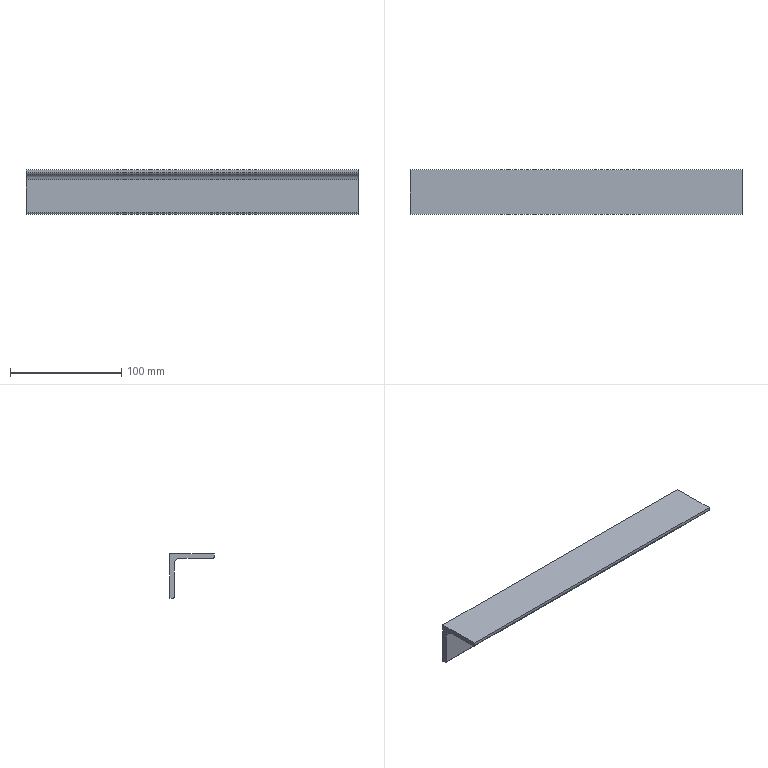Part | SolidWorks | features WeldMemberFeat 1, WeldmentFeature 1 | 1 solid | 11 faces | box 299 x 40 x 40 mm | volume 92272 mm3 | plane 8 | cylinder 3 | commonest cylinder face diameters 2.667 x2 10 x1
STEP:
#1=CARTESIAN_POINT('',(0.,-2.667,-40.));
#2=VERTEX_POINT('',#1);
#3=CARTESIAN_POINT('',(0.,0.,-40.));
#4=VERTEX_POINT('',#3);
#5=CARTESIAN_POINT('',(0.,0.,-40.));
#6=DIRECTION('',(0.,1.,0.));
#7=VECTOR('',#6,1000.);
#8=LINE('',#5,#7);
#9=EDGE_CURVE('',#2,#4,#8,.T.);
#10=ORIENTED_EDGE('',*,*,#9,.T.);
#11=CARTESIAN_POINT('',(299.,0.,-40.));
#12=VERTEX_POINT('',#11);
#13=CARTESIAN_POINT('',(299.,0.,-40.));
#14=DIRECTION('',(-1.,0.,0.));
#15=VECTOR('',#14,1000.);
#16=LINE('',#13,#15);
#17=EDGE_CURVE('',#12,#4,#16,.T.);
#18=ORIENTED_EDGE('',*,*,#17,.F.);
#19=CARTESIAN_POINT('',(299.,-2.667,-40.));
#20=VERTEX_POINT('',#19);
#21=CARTESIAN_POINT('',(299.,0.,-40.));
#22=DIRECTION('',(0.,1.,0.));
#23=VECTOR('',#22,1000.);
#24=LINE('',#21,#23);
#25=EDGE_CURVE('',#20,#12,#24,.T.);
#26=ORIENTED_EDGE('',*,*,#25,.F.);
#27=CARTESIAN_POINT('',(299.,-2.667,-40.));
#28=DIRECTION('',(-1.,0.,0.));
#29=VECTOR('',#28,1000.);
#30=LINE('',#27,#29);
#31=EDGE_CURVE('',#20,#2,#30,.T.);
#32=ORIENTED_EDGE('',*,*,#31,.T.);
#33=EDGE_LOOP('',(#10,#18,#26,#32));
#34=FACE_OUTER_BOUND('',#33,.T.);
#35=CARTESIAN_POINT('',(299.,0.,-40.));
#36=DIRECTION('',(0.,0.,1.));
#37=DIRECTION('',(0.,-1.,0.));
#38=AXIS2_PLACEMENT_3D('',#35,#36,#37);
#39=PLANE('',#38);
#40=ADVANCED_FACE('',(#34),#39,.F.);
#41=CARTESIAN_POINT('',(0.,0.,0.));
#42=VERTEX_POINT('',#41);
#43=CARTESIAN_POINT('',(0.,0.,-40.));
#44=DIRECTION('',(0.,0.,1.));
#45=VECTOR('',#44,1000.);
#46=LINE('',#43,#45);
#47=EDGE_CURVE('',#4,#42,#46,.T.);
#48=ORIENTED_EDGE('',*,*,#47,.T.);
#49=CARTESIAN_POINT('',(299.,0.,0.));
#50=VERTEX_POINT('',#49);
#51=CARTESIAN_POINT('',(299.,0.,0.));
#52=DIRECTION('',(-1.,0.,0.));
#53=VECTOR('',#52,1000.);
#54=LINE('',#51,#53);
#55=EDGE_CURVE('',#50,#42,#54,.T.);
#56=ORIENTED_EDGE('',*,*,#55,.F.);
#57=CARTESIAN_POINT('',(299.,0.,-40.));
#58=DIRECTION('',(0.,0.,1.));
#59=VECTOR('',#58,1000.);
#60=LINE('',#57,#59);
#61=EDGE_CURVE('',#12,#50,#60,.T.);
#62=ORIENTED_EDGE('',*,*,#61,.F.);
#63=ORIENTED_EDGE('',*,*,#17,.T.);
#64=EDGE_LOOP('',(#48,#56,#62,#63));
#65=FACE_OUTER_BOUND('',#64,.T.);
#66=CARTESIAN_POINT('',(299.,0.,-40.));
#67=DIRECTION('',(0.,-1.,0.));
#68=DIRECTION('',(0.,0.,-1.));
#69=AXIS2_PLACEMENT_3D('',#66,#67,#68);
#70=PLANE('',#69);
#71=ADVANCED_FACE('',(#65),#70,.F.);
#72=CARTESIAN_POINT('',(0.,-40.,0.));
#73=VERTEX_POINT('',#72);
#74=CARTESIAN_POINT('',(0.,0.,0.));
#75=DIRECTION('',(0.,-1.,0.));
#76=VECTOR('',#75,1000.);
#77=LINE('',#74,#76);
#78=EDGE_CURVE('',#42,#73,#77,.T.);
#79=ORIENTED_EDGE('',*,*,#78,.T.);
#80=CARTESIAN_POINT('',(299.,-40.,0.));
#81=VERTEX_POINT('',#80);
#82=CARTESIAN_POINT('',(299.,-40.,0.));
#83=DIRECTION('',(-1.,0.,0.));
#84=VECTOR('',#83,1000.);
#85=LINE('',#82,#84);
#86=EDGE_CURVE('',#81,#73,#85,.T.);
#87=ORIENTED_EDGE('',*,*,#86,.F.);
#88=CARTESIAN_POINT('',(299.,0.,0.));
#89=DIRECTION('',(0.,-1.,0.));
#90=VECTOR('',#89,1000.);
#91=LINE('',#88,#90);
#92=EDGE_CURVE('',#50,#81,#91,.T.);
#93=ORIENTED_EDGE('',*,*,#92,.F.);
#94=ORIENTED_EDGE('',*,*,#55,.T.);
#95=EDGE_LOOP('',(#79,#87,#93,#94));
#96=FACE_OUTER_BOUND('',#95,.T.);
#97=CARTESIAN_POINT('',(299.,0.,0.));
#98=DIRECTION('',(0.,0.,-1.));
#99=DIRECTION('',(0.,1.,0.));
#100=AXIS2_PLACEMENT_3D('',#97,#98,#99);
#101=PLANE('',#100);
#102=ADVANCED_FACE('',(#96),#101,.F.);
#103=CARTESIAN_POINT('',(0.,-40.,-2.667));
#104=VERTEX_POINT('',#103);
#105=CARTESIAN_POINT('',(0.,-40.,0.));
#106=DIRECTION('',(0.,0.,-1.));
#107=VECTOR('',#106,1000.);
#108=LINE('',#105,#107);
#109=EDGE_CURVE('',#73,#104,#108,.T.);
#110=ORIENTED_EDGE('',*,*,#109,.T.);
#111=CARTESIAN_POINT('',(299.,-40.,-2.667));
#112=VERTEX_POINT('',#111);
#113=CARTESIAN_POINT('',(299.,-40.,-2.667));
#114=DIRECTION('',(-1.,0.,0.));
#115=VECTOR('',#114,1000.);
#116=LINE('',#113,#115);
#117=EDGE_CURVE('',#112,#104,#116,.T.);
#118=ORIENTED_EDGE('',*,*,#117,.F.);
#119=CARTESIAN_POINT('',(299.,-40.,0.));
#120=DIRECTION('',(0.,0.,-1.));
#121=VECTOR('',#120,1000.);
#122=LINE('',#119,#121);
#123=EDGE_CURVE('',#81,#112,#122,.T.);
#124=ORIENTED_EDGE('',*,*,#123,.F.);
#125=ORIENTED_EDGE('',*,*,#86,.T.);
#126=EDGE_LOOP('',(#110,#118,#124,#125));
#127=FACE_OUTER_BOUND('',#126,.T.);
#128=CARTESIAN_POINT('',(299.,-40.,0.));
#129=DIRECTION('',(0.,1.,0.));
#130=DIRECTION('',(0.,0.,1.));
#131=AXIS2_PLACEMENT_3D('',#128,#129,#130);
#132=PLANE('',#131);
#133=ADVANCED_FACE('',(#127),#132,.F.);
#134=CARTESIAN_POINT('',(0.,-38.667,-4.));
#135=VERTEX_POINT('',#134);
#136=CARTESIAN_POINT('',(0.,-38.667,-2.667));
#137=DIRECTION('',(1.,0.,0.));
#138=DIRECTION('',(0.,0.,-1.));
#139=AXIS2_PLACEMENT_3D('',#136,#137,#138);
#140=CIRCLE('',#139,1.333);
#141=EDGE_CURVE('',#104,#135,#140,.T.);
#142=ORIENTED_EDGE('',*,*,#141,.T.);
#143=CARTESIAN_POINT('',(299.,-38.667,-4.));
#144=VERTEX_POINT('',#143);
#145=CARTESIAN_POINT('',(299.,-38.667,-4.));
#146=DIRECTION('',(-1.,0.,0.));
#147=VECTOR('',#146,1000.);
#148=LINE('',#145,#147);
#149=EDGE_CURVE('',#144,#135,#148,.T.);
#150=ORIENTED_EDGE('',*,*,#149,.F.);
#151=CARTESIAN_POINT('',(299.,-38.667,-2.667));
#152=DIRECTION('',(1.,0.,0.));
#153=DIRECTION('',(0.,0.,-1.));
#154=AXIS2_PLACEMENT_3D('',#151,#152,#153);
#155=CIRCLE('',#154,1.333);
#156=EDGE_CURVE('',#112,#144,#155,.T.);
#157=ORIENTED_EDGE('',*,*,#156,.F.);
#158=ORIENTED_EDGE('',*,*,#117,.T.);
#159=EDGE_LOOP('',(#142,#150,#157,#158));
#160=FACE_OUTER_BOUND('',#159,.T.);
#161=CARTESIAN_POINT('',(299.,-38.667,-2.667));
#162=DIRECTION('',(-1.,0.,0.));
#163=DIRECTION('',(0.,0.,1.));
#164=AXIS2_PLACEMENT_3D('',#161,#162,#163);
#165=CYLINDRICAL_SURFACE('',#164,1.333);
#166=ADVANCED_FACE('',(#160),#165,.T.);
#167=CARTESIAN_POINT('',(0.,-9.,-4.));
#168=VERTEX_POINT('',#167);
#169=CARTESIAN_POINT('',(0.,-9.,-4.));
#170=DIRECTION('',(0.,1.,0.));
#171=VECTOR('',#170,1000.);
#172=LINE('',#169,#171);
#173=EDGE_CURVE('',#135,#168,#172,.T.);
#174=ORIENTED_EDGE('',*,*,#173,.T.);
#175=CARTESIAN_POINT('',(299.,-9.,-4.));
#176=VERTEX_POINT('',#175);
#177=CARTESIAN_POINT('',(299.,-9.,-4.));
#178=DIRECTION('',(-1.,0.,0.));
#179=VECTOR('',#178,1000.);
#180=LINE('',#177,#179);
#181=EDGE_CURVE('',#176,#168,#180,.T.);
#182=ORIENTED_EDGE('',*,*,#181,.F.);
#183=CARTESIAN_POINT('',(299.,-9.,-4.));
#184=DIRECTION('',(0.,1.,0.));
#185=VECTOR('',#184,1000.);
#186=LINE('',#183,#185);
#187=EDGE_CURVE('',#144,#176,#186,.T.);
#188=ORIENTED_EDGE('',*,*,#187,.F.);
#189=ORIENTED_EDGE('',*,*,#149,.T.);
#190=EDGE_LOOP('',(#174,#182,#188,#189));
#191=FACE_OUTER_BOUND('',#190,.T.);
#192=CARTESIAN_POINT('',(299.,-9.,-4.));
#193=DIRECTION('',(0.,0.,1.));
#194=DIRECTION('',(0.,-1.,0.));
#195=AXIS2_PLACEMENT_3D('',#192,#193,#194);
#196=PLANE('',#195);
#197=ADVANCED_FACE('',(#191),#196,.F.);
#198=CARTESIAN_POINT('',(0.,-4.,-9.));
#199=VERTEX_POINT('',#198);
#200=CARTESIAN_POINT('',(0.,-9.,-9.));
#201=DIRECTION('',(-1.,0.,0.));
#202=DIRECTION('',(0.,0.,-1.));
#203=AXIS2_PLACEMENT_3D('',#200,#201,#202);
#204=CIRCLE('',#203,5.);
#205=EDGE_CURVE('',#168,#199,#204,.T.);
#206=ORIENTED_EDGE('',*,*,#205,.T.);
#207=CARTESIAN_POINT('',(299.,-4.,-9.));
#208=VERTEX_POINT('',#207);
#209=CARTESIAN_POINT('',(299.,-4.,-9.));
#210=DIRECTION('',(-1.,0.,0.));
#211=VECTOR('',#210,1000.);
#212=LINE('',#209,#211);
#213=EDGE_CURVE('',#208,#199,#212,.T.);
#214=ORIENTED_EDGE('',*,*,#213,.F.);
#215=CARTESIAN_POINT('',(299.,-9.,-9.));
#216=DIRECTION('',(-1.,0.,0.));
#217=DIRECTION('',(0.,0.,-1.));
#218=AXIS2_PLACEMENT_3D('',#215,#216,#217);
#219=CIRCLE('',#218,5.);
#220=EDGE_CURVE('',#176,#208,#219,.T.);
#221=ORIENTED_EDGE('',*,*,#220,.F.);
#222=ORIENTED_EDGE('',*,*,#181,.T.);
#223=EDGE_LOOP('',(#206,#214,#221,#222));
#224=FACE_OUTER_BOUND('',#223,.T.);
#225=CARTESIAN_POINT('',(299.,-9.,-9.));
#226=DIRECTION('',(-1.,0.,0.));
#227=DIRECTION('',(0.,0.,1.));
#228=AXIS2_PLACEMENT_3D('',#225,#226,#227);
#229=CYLINDRICAL_SURFACE('',#228,5.);
#230=ADVANCED_FACE('',(#224),#229,.F.);
#231=CARTESIAN_POINT('',(0.,-4.,-38.667));
#232=VERTEX_POINT('',#231);
#233=CARTESIAN_POINT('',(0.,-4.,-38.667));
#234=DIRECTION('',(0.,0.,-1.));
#235=VECTOR('',#234,1000.);
#236=LINE('',#233,#235);
#237=EDGE_CURVE('',#199,#232,#236,.T.);
#238=ORIENTED_EDGE('',*,*,#237,.T.);
#239=CARTESIAN_POINT('',(299.,-4.,-38.667));
#240=VERTEX_POINT('',#239);
#241=CARTESIAN_POINT('',(299.,-4.,-38.667));
#242=DIRECTION('',(-1.,0.,0.));
#243=VECTOR('',#242,1000.);
#244=LINE('',#241,#243);
#245=EDGE_CURVE('',#240,#232,#244,.T.);
#246=ORIENTED_EDGE('',*,*,#245,.F.);
#247=CARTESIAN_POINT('',(299.,-4.,-38.667));
#248=DIRECTION('',(0.,0.,-1.));
#249=VECTOR('',#248,1000.);
#250=LINE('',#247,#249);
#251=EDGE_CURVE('',#208,#240,#250,.T.);
#252=ORIENTED_EDGE('',*,*,#251,.F.);
#253=ORIENTED_EDGE('',*,*,#213,.T.);
#254=EDGE_LOOP('',(#238,#246,#252,#253));
#255=FACE_OUTER_BOUND('',#254,.T.);
#256=CARTESIAN_POINT('',(299.,-4.,-38.667));
#257=DIRECTION('',(0.,1.,0.));
#258=DIRECTION('',(0.,0.,1.));
#259=AXIS2_PLACEMENT_3D('',#256,#257,#258);
#260=PLANE('',#259);
#261=ADVANCED_FACE('',(#255),#260,.F.);
#262=CARTESIAN_POINT('',(0.,-2.667,-38.667));
#263=DIRECTION('',(1.,0.,0.));
#264=DIRECTION('',(0.,0.,1.));
#265=AXIS2_PLACEMENT_3D('',#262,#263,#264);
#266=CIRCLE('',#265,1.333);
#267=EDGE_CURVE('',#232,#2,#266,.T.);
#268=ORIENTED_EDGE('',*,*,#267,.T.);
#269=ORIENTED_EDGE('',*,*,#31,.F.);
#270=CARTESIAN_POINT('',(299.,-2.667,-38.667));
#271=DIRECTION('',(1.,0.,0.));
#272=DIRECTION('',(0.,0.,1.));
#273=AXIS2_PLACEMENT_3D('',#270,#271,#272);
#274=CIRCLE('',#273,1.333);
#275=EDGE_CURVE('',#240,#20,#274,.T.);
#276=ORIENTED_EDGE('',*,*,#275,.F.);
#277=ORIENTED_EDGE('',*,*,#245,.T.);
#278=EDGE_LOOP('',(#268,#269,#276,#277));
#279=FACE_OUTER_BOUND('',#278,.T.);
#280=CARTESIAN_POINT('',(299.,-2.667,-38.667));
#281=DIRECTION('',(-1.,0.,0.));
#282=DIRECTION('',(0.,0.,1.));
#283=AXIS2_PLACEMENT_3D('',#280,#281,#282);
#284=CYLINDRICAL_SURFACE('',#283,1.333);
#285=ADVANCED_FACE('',(#279),#284,.T.);
#286=ORIENTED_EDGE('',*,*,#25,.T.);
#287=ORIENTED_EDGE('',*,*,#61,.T.);
#288=ORIENTED_EDGE('',*,*,#92,.T.);
#289=ORIENTED_EDGE('',*,*,#123,.T.);
#290=ORIENTED_EDGE('',*,*,#156,.T.);
#291=ORIENTED_EDGE('',*,*,#187,.T.);
#292=ORIENTED_EDGE('',*,*,#220,.T.);
#293=ORIENTED_EDGE('',*,*,#251,.T.);
#294=ORIENTED_EDGE('',*,*,#275,.T.);
#295=EDGE_LOOP('',(#286,#287,#288,#289,#290,#291,#292,#293,#294));
#296=FACE_OUTER_BOUND('',#295,.T.);
#297=CARTESIAN_POINT('',(299.,-2.667,-38.667));
#298=DIRECTION('',(-1.,0.,0.));
#299=DIRECTION('',(0.,0.,1.));
#300=AXIS2_PLACEMENT_3D('',#297,#298,#299);
#301=PLANE('',#300);
#302=ADVANCED_FACE('',(#296),#301,.F.);
#303=ORIENTED_EDGE('',*,*,#9,.F.);
#304=ORIENTED_EDGE('',*,*,#267,.F.);
#305=ORIENTED_EDGE('',*,*,#237,.F.);
#306=ORIENTED_EDGE('',*,*,#205,.F.);
#307=ORIENTED_EDGE('',*,*,#173,.F.);
#308=ORIENTED_EDGE('',*,*,#141,.F.);
#309=ORIENTED_EDGE('',*,*,#109,.F.);
#310=ORIENTED_EDGE('',*,*,#78,.F.);
#311=ORIENTED_EDGE('',*,*,#47,.F.);
#312=EDGE_LOOP('',(#303,#304,#305,#306,#307,#308,#309,#310,#311));
#313=FACE_OUTER_BOUND('',#312,.T.);
#314=CARTESIAN_POINT('',(0.,-2.667,-38.667));
#315=DIRECTION('',(-1.,0.,0.));
#316=DIRECTION('',(0.,0.,1.));
#317=AXIS2_PLACEMENT_3D('',#314,#315,#316);
#318=PLANE('',#317);
#319=ADVANCED_FACE('',(#313),#318,.T.);
#320=CLOSED_SHELL('',(#40,#71,#102,#133,#166,#197,#230,#261,#285,#302,#319));
#321=MANIFOLD_SOLID_BREP('',#320);
#322=CARTESIAN_POINT('',(0.,0.,0.));
#323=DIRECTION('',(0.,0.,1.));
#324=DIRECTION('',(1.,0.,0.));
#325=AXIS2_PLACEMENT_3D('',#322,#323,#324);
#326=(LENGTH_UNIT()NAMED_UNIT(*)SI_UNIT(.MILLI.,.METRE.));
#327=UNCERTAINTY_MEASURE_WITH_UNIT(LENGTH_MEASURE(0.00001),#326,'','');
#328=(NAMED_UNIT(*)PLANE_ANGLE_UNIT()SI_UNIT($,.RADIAN.));
#329=(NAMED_UNIT(*)SI_UNIT($,.STERADIAN.)SOLID_ANGLE_UNIT());
#330=(GEOMETRIC_REPRESENTATION_CONTEXT(3)GLOBAL_UNCERTAINTY_ASSIGNED_CONTEXT((#327))GLOBAL_UNIT_ASSIGNED_CONTEXT((#326,#328,#329))REPRESENTATION_CONTEXT('',''));
#331=ADVANCED_BREP_SHAPE_REPRESENTATION('',(#321,#325),#330);